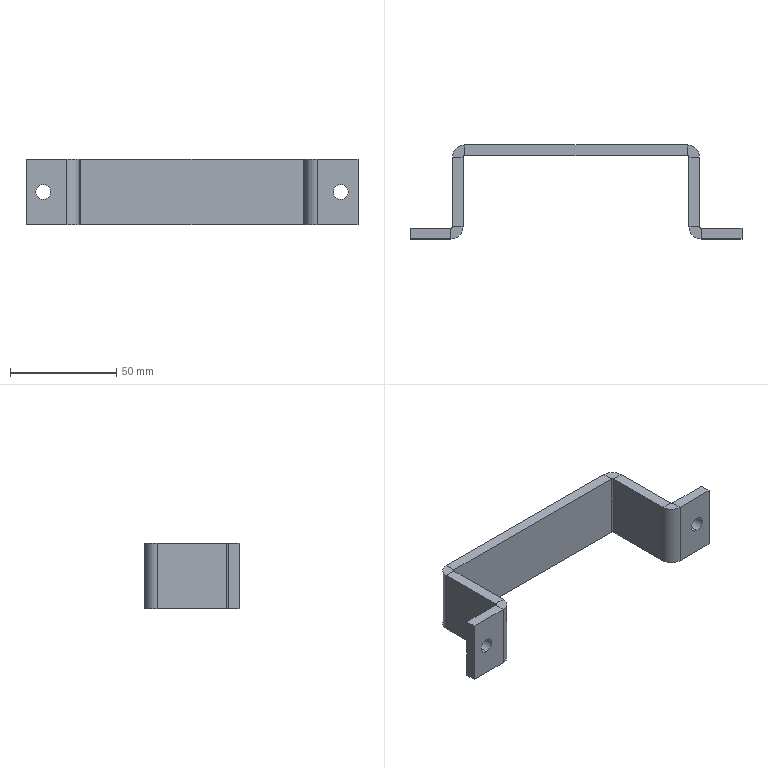Part | SolidWorks | features FlatPattern 1, ICE 1, SMBaseFlange 1, SheetMetal 1 | 1 solid | 42 faces | box 156.25 x 44.25 x 30.75 mm | volume 34854 mm3 | plane 30 | cylinder 12 | commonest cylinder face diameters 1.473 x4 7 x4 11.473 x4
STEP:
#1=CARTESIAN_POINT('',(-70.,-44.25,3.5));
#2=VERTEX_POINT('',#1);
#3=CARTESIAN_POINT('',(-70.,-44.25,-3.5));
#4=VERTEX_POINT('',#3);
#5=CARTESIAN_POINT('',(-70.,-44.25,0.));
#6=DIRECTION('',(0.,-1.,0.));
#7=DIRECTION('',(0.,0.,-1.));
#8=AXIS2_PLACEMENT_3D('',#5,#6,#7);
#9=CIRCLE('',#8,3.5);
#10=EDGE_CURVE('',#2,#4,#9,.T.);
#11=ORIENTED_EDGE('',*,*,#10,.T.);
#12=CARTESIAN_POINT('',(-70.,-39.25,-3.5));
#13=VERTEX_POINT('',#12);
#14=CARTESIAN_POINT('',(-70.,-49.25,-3.5));
#15=DIRECTION('',(0.,1.,0.));
#16=VECTOR('',#15,1000.);
#17=LINE('',#14,#16);
#18=EDGE_CURVE('',#4,#13,#17,.T.);
#19=ORIENTED_EDGE('',*,*,#18,.T.);
#20=CARTESIAN_POINT('',(-70.,-39.25,3.5));
#21=VERTEX_POINT('',#20);
#22=CARTESIAN_POINT('',(-70.,-39.25,0.));
#23=DIRECTION('',(0.,1.,0.));
#24=DIRECTION('',(0.,0.,1.));
#25=AXIS2_PLACEMENT_3D('',#22,#23,#24);
#26=CIRCLE('',#25,3.5);
#27=EDGE_CURVE('',#13,#21,#26,.T.);
#28=ORIENTED_EDGE('',*,*,#27,.T.);
#29=CARTESIAN_POINT('',(-70.,-49.25,3.5));
#30=DIRECTION('',(0.,1.,0.));
#31=VECTOR('',#30,1000.);
#32=LINE('',#29,#31);
#33=EDGE_CURVE('',#2,#21,#32,.T.);
#34=ORIENTED_EDGE('',*,*,#33,.F.);
#35=EDGE_LOOP('',(#11,#19,#28,#34));
#36=FACE_OUTER_BOUND('',#35,.T.);
#37=CARTESIAN_POINT('',(-70.,-49.25,0.));
#38=DIRECTION('',(0.,1.,0.));
#39=DIRECTION('',(0.,0.,1.));
#40=AXIS2_PLACEMENT_3D('',#37,#38,#39);
#41=CYLINDRICAL_SURFACE('',#40,3.5);
#42=ADVANCED_FACE('',(#36),#41,.F.);
#43=CARTESIAN_POINT('',(70.,-44.25,3.5));
#44=VERTEX_POINT('',#43);
#45=CARTESIAN_POINT('',(70.,-44.25,-3.5));
#46=VERTEX_POINT('',#45);
#47=CARTESIAN_POINT('',(70.,-44.25,0.));
#48=DIRECTION('',(0.,-1.,0.));
#49=DIRECTION('',(0.,0.,-1.));
#50=AXIS2_PLACEMENT_3D('',#47,#48,#49);
#51=CIRCLE('',#50,3.5);
#52=EDGE_CURVE('',#44,#46,#51,.T.);
#53=ORIENTED_EDGE('',*,*,#52,.T.);
#54=CARTESIAN_POINT('',(70.,-39.25,-3.5));
#55=VERTEX_POINT('',#54);
#56=CARTESIAN_POINT('',(70.,-49.25,-3.5));
#57=DIRECTION('',(0.,1.,0.));
#58=VECTOR('',#57,1000.);
#59=LINE('',#56,#58);
#60=EDGE_CURVE('',#46,#55,#59,.T.);
#61=ORIENTED_EDGE('',*,*,#60,.T.);
#62=CARTESIAN_POINT('',(70.,-39.25,3.5));
#63=VERTEX_POINT('',#62);
#64=CARTESIAN_POINT('',(70.,-39.25,0.));
#65=DIRECTION('',(0.,1.,0.));
#66=DIRECTION('',(0.,0.,1.));
#67=AXIS2_PLACEMENT_3D('',#64,#65,#66);
#68=CIRCLE('',#67,3.5);
#69=EDGE_CURVE('',#55,#63,#68,.T.);
#70=ORIENTED_EDGE('',*,*,#69,.T.);
#71=CARTESIAN_POINT('',(70.,-49.25,3.5));
#72=DIRECTION('',(0.,1.,0.));
#73=VECTOR('',#72,1000.);
#74=LINE('',#71,#73);
#75=EDGE_CURVE('',#44,#63,#74,.T.);
#76=ORIENTED_EDGE('',*,*,#75,.F.);
#77=EDGE_LOOP('',(#53,#61,#70,#76));
#78=FACE_OUTER_BOUND('',#77,.T.);
#79=CARTESIAN_POINT('',(70.,-49.25,0.));
#80=DIRECTION('',(0.,1.,0.));
#81=DIRECTION('',(0.,0.,1.));
#82=AXIS2_PLACEMENT_3D('',#79,#80,#81);
#83=CYLINDRICAL_SURFACE('',#82,3.5);
#84=ADVANCED_FACE('',(#78),#83,.F.);
#85=CARTESIAN_POINT('',(58.862,-39.25,15.375));
#86=VERTEX_POINT('',#85);
#87=CARTESIAN_POINT('',(58.862,-44.25,15.375));
#88=VERTEX_POINT('',#87);
#89=CARTESIAN_POINT('',(58.862,-39.25,15.375));
#90=DIRECTION('',(0.,-1.,0.));
#91=VECTOR('',#90,1000.);
#92=LINE('',#89,#91);
#93=EDGE_CURVE('',#86,#88,#92,.T.);
#94=ORIENTED_EDGE('',*,*,#93,.F.);
#95=CARTESIAN_POINT('',(58.125,-38.513,15.375));
#96=VERTEX_POINT('',#95);
#97=CARTESIAN_POINT('',(58.862,-38.513,15.375));
#98=DIRECTION('',(0.,0.,-1.));
#99=DIRECTION('',(1.,0.,0.));
#100=AXIS2_PLACEMENT_3D('',#97,#98,#99);
#101=CIRCLE('',#100,0.7366);
#102=EDGE_CURVE('',#86,#96,#101,.T.);
#103=ORIENTED_EDGE('',*,*,#102,.T.);
#104=CARTESIAN_POINT('',(53.125,-38.513,15.375));
#105=VERTEX_POINT('',#104);
#106=CARTESIAN_POINT('',(53.125,-38.513,15.375));
#107=DIRECTION('',(1.,0.,0.));
#108=VECTOR('',#107,1000.);
#109=LINE('',#106,#108);
#110=EDGE_CURVE('',#105,#96,#109,.T.);
#111=ORIENTED_EDGE('',*,*,#110,.F.);
#112=CARTESIAN_POINT('',(58.862,-38.513,15.375));
#113=DIRECTION('',(0.,0.,-1.));
#114=DIRECTION('',(1.,0.,0.));
#115=AXIS2_PLACEMENT_3D('',#112,#113,#114);
#116=CIRCLE('',#115,5.737);
#117=EDGE_CURVE('',#88,#105,#116,.T.);
#118=ORIENTED_EDGE('',*,*,#117,.F.);
#119=EDGE_LOOP('',(#94,#103,#111,#118));
#120=FACE_OUTER_BOUND('',#119,.T.);
#121=CARTESIAN_POINT('',(58.862,-39.25,15.375));
#122=DIRECTION('',(0.,0.,1.));
#123=DIRECTION('',(1.,0.,0.));
#124=AXIS2_PLACEMENT_3D('',#121,#122,#123);
#125=PLANE('',#124);
#126=ADVANCED_FACE('',(#120),#125,.T.);
#127=CARTESIAN_POINT('',(78.125,-39.25,15.375));
#128=VERTEX_POINT('',#127);
#129=CARTESIAN_POINT('',(58.125,-39.25,15.375));
#130=DIRECTION('',(-1.,0.,0.));
#131=VECTOR('',#130,1000.);
#132=LINE('',#129,#131);
#133=EDGE_CURVE('',#128,#86,#132,.T.);
#134=ORIENTED_EDGE('',*,*,#133,.T.);
#135=ORIENTED_EDGE('',*,*,#93,.T.);
#136=CARTESIAN_POINT('',(78.125,-44.25,15.375));
#137=VERTEX_POINT('',#136);
#138=CARTESIAN_POINT('',(58.125,-44.25,15.375));
#139=DIRECTION('',(-1.,0.,0.));
#140=VECTOR('',#139,1000.);
#141=LINE('',#138,#140);
#142=EDGE_CURVE('',#137,#88,#141,.T.);
#143=ORIENTED_EDGE('',*,*,#142,.F.);
#144=CARTESIAN_POINT('',(78.125,-39.25,15.375));
#145=DIRECTION('',(0.,-1.,0.));
#146=VECTOR('',#145,1000.);
#147=LINE('',#144,#146);
#148=EDGE_CURVE('',#128,#137,#147,.T.);
#149=ORIENTED_EDGE('',*,*,#148,.F.);
#150=EDGE_LOOP('',(#134,#135,#143,#149));
#151=FACE_OUTER_BOUND('',#150,.T.);
#152=CARTESIAN_POINT('',(53.125,-38.513,15.375));
#153=DIRECTION('',(0.,0.,1.));
#154=DIRECTION('',(1.,0.,0.));
#155=AXIS2_PLACEMENT_3D('',#152,#153,#154);
#156=PLANE('',#155);
#157=ADVANCED_FACE('',(#151),#156,.T.);
#158=CARTESIAN_POINT('',(58.125,-38.513,-15.375));
#159=VERTEX_POINT('',#158);
#160=CARTESIAN_POINT('',(53.125,-38.513,-15.375));
#161=VERTEX_POINT('',#160);
#162=CARTESIAN_POINT('',(58.125,-38.513,-15.375));
#163=DIRECTION('',(-1.,0.,0.));
#164=VECTOR('',#163,1000.);
#165=LINE('',#162,#164);
#166=EDGE_CURVE('',#159,#161,#165,.T.);
#167=ORIENTED_EDGE('',*,*,#166,.F.);
#168=CARTESIAN_POINT('',(58.862,-39.25,-15.375));
#169=VERTEX_POINT('',#168);
#170=CARTESIAN_POINT('',(58.862,-38.513,-15.375));
#171=DIRECTION('',(0.,0.,-1.));
#172=DIRECTION('',(1.,0.,0.));
#173=AXIS2_PLACEMENT_3D('',#170,#171,#172);
#174=CIRCLE('',#173,0.7366);
#175=EDGE_CURVE('',#169,#159,#174,.T.);
#176=ORIENTED_EDGE('',*,*,#175,.F.);
#177=CARTESIAN_POINT('',(58.862,-44.25,-15.375));
#178=VERTEX_POINT('',#177);
#179=CARTESIAN_POINT('',(58.862,-44.25,-15.375));
#180=DIRECTION('',(0.,1.,0.));
#181=VECTOR('',#180,1000.);
#182=LINE('',#179,#181);
#183=EDGE_CURVE('',#178,#169,#182,.T.);
#184=ORIENTED_EDGE('',*,*,#183,.F.);
#185=CARTESIAN_POINT('',(58.862,-38.513,-15.375));
#186=DIRECTION('',(0.,0.,-1.));
#187=DIRECTION('',(1.,0.,0.));
#188=AXIS2_PLACEMENT_3D('',#185,#186,#187);
#189=CIRCLE('',#188,5.737);
#190=EDGE_CURVE('',#178,#161,#189,.T.);
#191=ORIENTED_EDGE('',*,*,#190,.T.);
#192=EDGE_LOOP('',(#167,#176,#184,#191));
#193=FACE_OUTER_BOUND('',#192,.T.);
#194=CARTESIAN_POINT('',(58.125,-38.513,-15.375));
#195=DIRECTION('',(0.,0.,-1.));
#196=DIRECTION('',(-1.,0.,0.));
#197=AXIS2_PLACEMENT_3D('',#194,#195,#196);
#198=PLANE('',#197);
#199=ADVANCED_FACE('',(#193),#198,.T.);
#200=CARTESIAN_POINT('',(58.125,-5.737,-15.375));
#201=VERTEX_POINT('',#200);
#202=CARTESIAN_POINT('',(58.125,0.,-15.375));
#203=DIRECTION('',(0.,1.,0.));
#204=VECTOR('',#203,1000.);
#205=LINE('',#202,#204);
#206=EDGE_CURVE('',#159,#201,#205,.T.);
#207=ORIENTED_EDGE('',*,*,#206,.F.);
#208=ORIENTED_EDGE('',*,*,#166,.T.);
#209=CARTESIAN_POINT('',(53.125,-5.737,-15.375));
#210=VERTEX_POINT('',#209);
#211=CARTESIAN_POINT('',(53.125,0.,-15.375));
#212=DIRECTION('',(0.,1.,0.));
#213=VECTOR('',#212,1000.);
#214=LINE('',#211,#213);
#215=EDGE_CURVE('',#161,#210,#214,.T.);
#216=ORIENTED_EDGE('',*,*,#215,.T.);
#217=CARTESIAN_POINT('',(53.125,-5.737,-15.375));
#218=DIRECTION('',(1.,0.,0.));
#219=VECTOR('',#218,1000.);
#220=LINE('',#217,#219);
#221=EDGE_CURVE('',#210,#201,#220,.T.);
#222=ORIENTED_EDGE('',*,*,#221,.T.);
#223=EDGE_LOOP('',(#207,#208,#216,#222));
#224=FACE_OUTER_BOUND('',#223,.T.);
#225=CARTESIAN_POINT('',(58.862,-44.25,-15.375));
#226=DIRECTION('',(0.,0.,-1.));
#227=DIRECTION('',(-1.,0.,0.));
#228=AXIS2_PLACEMENT_3D('',#225,#226,#227);
#229=PLANE('',#228);
#230=ADVANCED_FACE('',(#224),#229,.T.);
#231=CARTESIAN_POINT('',(58.125,-5.737,15.375));
#232=VERTEX_POINT('',#231);
#233=CARTESIAN_POINT('',(53.125,-5.737,15.375));
#234=VERTEX_POINT('',#233);
#235=CARTESIAN_POINT('',(58.125,-5.737,15.375));
#236=DIRECTION('',(-1.,0.,0.));
#237=VECTOR('',#236,1000.);
#238=LINE('',#235,#237);
#239=EDGE_CURVE('',#232,#234,#238,.T.);
#240=ORIENTED_EDGE('',*,*,#239,.F.);
#241=CARTESIAN_POINT('',(52.388,0.,15.375));
#242=VERTEX_POINT('',#241);
#243=CARTESIAN_POINT('',(52.388,-5.737,15.375));
#244=DIRECTION('',(0.,0.,1.));
#245=DIRECTION('',(-1.,0.,0.));
#246=AXIS2_PLACEMENT_3D('',#243,#244,#245);
#247=CIRCLE('',#246,5.737);
#248=EDGE_CURVE('',#232,#242,#247,.T.);
#249=ORIENTED_EDGE('',*,*,#248,.T.);
#250=CARTESIAN_POINT('',(52.388,-5.,15.375));
#251=VERTEX_POINT('',#250);
#252=CARTESIAN_POINT('',(52.388,-5.,15.375));
#253=DIRECTION('',(0.,1.,0.));
#254=VECTOR('',#253,1000.);
#255=LINE('',#252,#254);
#256=EDGE_CURVE('',#251,#242,#255,.T.);
#257=ORIENTED_EDGE('',*,*,#256,.F.);
#258=CARTESIAN_POINT('',(52.388,-5.737,15.375));
#259=DIRECTION('',(0.,0.,1.));
#260=DIRECTION('',(1.,0.,0.));
#261=AXIS2_PLACEMENT_3D('',#258,#259,#260);
#262=CIRCLE('',#261,0.7366);
#263=EDGE_CURVE('',#234,#251,#262,.T.);
#264=ORIENTED_EDGE('',*,*,#263,.F.);
#265=EDGE_LOOP('',(#240,#249,#257,#264));
#266=FACE_OUTER_BOUND('',#265,.T.);
#267=CARTESIAN_POINT('',(58.125,-5.737,15.375));
#268=DIRECTION('',(0.,0.,1.));
#269=DIRECTION('',(1.,0.,0.));
#270=AXIS2_PLACEMENT_3D('',#267,#268,#269);
#271=PLANE('',#270);
#272=ADVANCED_FACE('',(#266),#271,.T.);
#273=CARTESIAN_POINT('',(58.125,0.,15.375));
#274=DIRECTION('',(0.,1.,0.));
#275=VECTOR('',#274,1000.);
#276=LINE('',#273,#275);
#277=EDGE_CURVE('',#96,#232,#276,.T.);
#278=ORIENTED_EDGE('',*,*,#277,.T.);
#279=ORIENTED_EDGE('',*,*,#239,.T.);
#280=CARTESIAN_POINT('',(53.125,0.,15.375));
#281=DIRECTION('',(0.,1.,0.));
#282=VECTOR('',#281,1000.);
#283=LINE('',#280,#282);
#284=EDGE_CURVE('',#105,#234,#283,.T.);
#285=ORIENTED_EDGE('',*,*,#284,.F.);
#286=ORIENTED_EDGE('',*,*,#110,.T.);
#287=EDGE_LOOP('',(#278,#279,#285,#286));
#288=FACE_OUTER_BOUND('',#287,.T.);
#289=CARTESIAN_POINT('',(52.388,-5.,15.375));
#290=DIRECTION('',(0.,0.,1.));
#291=DIRECTION('',(1.,0.,0.));
#292=AXIS2_PLACEMENT_3D('',#289,#290,#291);
#293=PLANE('',#292);
#294=ADVANCED_FACE('',(#288),#293,.T.);
#295=CARTESIAN_POINT('',(52.388,0.,-15.375));
#296=VERTEX_POINT('',#295);
#297=CARTESIAN_POINT('',(52.388,-5.,-15.375));
#298=VERTEX_POINT('',#297);
#299=CARTESIAN_POINT('',(52.388,0.,-15.375));
#300=DIRECTION('',(0.,-1.,0.));
#301=VECTOR('',#300,1000.);
#302=LINE('',#299,#301);
#303=EDGE_CURVE('',#296,#298,#302,.T.);
#304=ORIENTED_EDGE('',*,*,#303,.F.);
#305=CARTESIAN_POINT('',(52.388,-5.737,-15.375));
#306=DIRECTION('',(0.,0.,1.));
#307=DIRECTION('',(-1.,0.,0.));
#308=AXIS2_PLACEMENT_3D('',#305,#306,#307);
#309=CIRCLE('',#308,5.737);
#310=EDGE_CURVE('',#201,#296,#309,.T.);
#311=ORIENTED_EDGE('',*,*,#310,.F.);
#312=ORIENTED_EDGE('',*,*,#221,.F.);
#313=CARTESIAN_POINT('',(52.388,-5.737,-15.375));
#314=DIRECTION('',(0.,0.,1.));
#315=DIRECTION('',(1.,0.,0.));
#316=AXIS2_PLACEMENT_3D('',#313,#314,#315);
#317=CIRCLE('',#316,0.7366);
#318=EDGE_CURVE('',#210,#298,#317,.T.);
#319=ORIENTED_EDGE('',*,*,#318,.T.);
#320=EDGE_LOOP('',(#304,#311,#312,#319));
#321=FACE_OUTER_BOUND('',#320,.T.);
#322=CARTESIAN_POINT('',(52.388,0.,-15.375));
#323=DIRECTION('',(0.,0.,-1.));
#324=DIRECTION('',(-1.,0.,0.));
#325=AXIS2_PLACEMENT_3D('',#322,#323,#324);
#326=PLANE('',#325);
#327=ADVANCED_FACE('',(#321),#326,.T.);
#328=CARTESIAN_POINT('',(-52.388,0.,-15.375));
#329=VERTEX_POINT('',#328);
#330=CARTESIAN_POINT('',(-58.125,0.,-15.375));
#331=DIRECTION('',(-1.,0.,0.));
#332=VECTOR('',#331,1000.);
#333=LINE('',#330,#332);
#334=EDGE_CURVE('',#296,#329,#333,.T.);
#335=ORIENTED_EDGE('',*,*,#334,.F.);
#336=ORIENTED_EDGE('',*,*,#303,.T.);
#337=CARTESIAN_POINT('',(-52.388,-5.,-15.375));
#338=VERTEX_POINT('',#337);
#339=CARTESIAN_POINT('',(-58.125,-5.,-15.375));
#340=DIRECTION('',(-1.,0.,0.));
#341=VECTOR('',#340,1000.);
#342=LINE('',#339,#341);
#343=EDGE_CURVE('',#298,#338,#342,.T.);
#344=ORIENTED_EDGE('',*,*,#343,.T.);
#345=CARTESIAN_POINT('',(-52.388,-5.,-15.375));
#346=DIRECTION('',(0.,1.,0.));
#347=VECTOR('',#346,1000.);
#348=LINE('',#345,#347);
#349=EDGE_CURVE('',#338,#329,#348,.T.);
#350=ORIENTED_EDGE('',*,*,#349,.T.);
#351=EDGE_LOOP('',(#335,#336,#344,#350));
#352=FACE_OUTER_BOUND('',#351,.T.);
#353=CARTESIAN_POINT('',(53.125,-5.737,-15.375));
#354=DIRECTION('',(0.,0.,-1.));
#355=DIRECTION('',(-1.,0.,0.));
#356=AXIS2_PLACEMENT_3D('',#353,#354,#355);
#357=PLANE('',#356);
#358=ADVANCED_FACE('',(#352),#357,.T.);
#359=CARTESIAN_POINT('',(-52.388,0.,15.375));
#360=VERTEX_POINT('',#359);
#361=CARTESIAN_POINT('',(-52.388,-5.,15.375));
#362=VERTEX_POINT('',#361);
#363=CARTESIAN_POINT('',(-52.388,0.,15.375));
#364=DIRECTION('',(0.,-1.,0.));
#365=VECTOR('',#364,1000.);
#366=LINE('',#363,#365);
#367=EDGE_CURVE('',#360,#362,#366,.T.);
#368=ORIENTED_EDGE('',*,*,#367,.F.);
#369=CARTESIAN_POINT('',(-58.125,-5.737,15.375));
#370=VERTEX_POINT('',#369);
#371=CARTESIAN_POINT('',(-52.388,-5.737,15.375));
#372=DIRECTION('',(0.,0.,1.));
#373=DIRECTION('',(-1.,0.,0.));
#374=AXIS2_PLACEMENT_3D('',#371,#372,#373);
#375=CIRCLE('',#374,5.737);
#376=EDGE_CURVE('',#360,#370,#375,.T.);
#377=ORIENTED_EDGE('',*,*,#376,.T.);
#378=CARTESIAN_POINT('',(-53.125,-5.737,15.375));
#379=VERTEX_POINT('',#378);
#380=CARTESIAN_POINT('',(-53.125,-5.737,15.375));
#381=DIRECTION('',(-1.,0.,0.));
#382=VECTOR('',#381,1000.);
#383=LINE('',#380,#382);
#384=EDGE_CURVE('',#379,#370,#383,.T.);
#385=ORIENTED_EDGE('',*,*,#384,.F.);
#386=CARTESIAN_POINT('',(-52.388,-5.737,15.375));
#387=DIRECTION('',(0.,0.,1.));
#388=DIRECTION('',(1.,0.,0.));
#389=AXIS2_PLACEMENT_3D('',#386,#387,#388);
#390=CIRCLE('',#389,0.7366);
#391=EDGE_CURVE('',#362,#379,#390,.T.);
#392=ORIENTED_EDGE('',*,*,#391,.F.);
#393=EDGE_LOOP('',(#368,#377,#385,#392));
#394=FACE_OUTER_BOUND('',#393,.T.);
#395=CARTESIAN_POINT('',(-52.388,0.,15.375));
#396=DIRECTION('',(0.,0.,1.));
#397=DIRECTION('',(1.,0.,0.));
#398=AXIS2_PLACEMENT_3D('',#395,#396,#397);
#399=PLANE('',#398);
#400=ADVANCED_FACE('',(#394),#399,.T.);
#401=CARTESIAN_POINT('',(-58.125,0.,15.375));
#402=DIRECTION('',(-1.,0.,0.));
#403=VECTOR('',#402,1000.);
#404=LINE('',#401,#403);
#405=EDGE_CURVE('',#242,#360,#404,.T.);
#406=ORIENTED_EDGE('',*,*,#405,.T.);
#407=ORIENTED_EDGE('',*,*,#367,.T.);
#408=CARTESIAN_POINT('',(-58.125,-5.,15.375));
#409=DIRECTION('',(-1.,0.,0.));
#410=VECTOR('',#409,1000.);
#411=LINE('',#408,#410);
#412=EDGE_CURVE('',#251,#362,#411,.T.);
#413=ORIENTED_EDGE('',*,*,#412,.F.);
#414=ORIENTED_EDGE('',*,*,#256,.T.);
#415=EDGE_LOOP('',(#406,#407,#413,#414));
#416=FACE_OUTER_BOUND('',#415,.T.);
#417=CARTESIAN_POINT('',(-53.125,-5.737,15.375));
#418=DIRECTION('',(0.,0.,1.));
#419=DIRECTION('',(1.,0.,0.));
#420=AXIS2_PLACEMENT_3D('',#417,#418,#419);
#421=PLANE('',#420);
#422=ADVANCED_FACE('',(#416),#421,.T.);
#423=CARTESIAN_POINT('',(-58.125,-5.737,-15.375));
#424=VERTEX_POINT('',#423);
#425=CARTESIAN_POINT('',(-53.125,-5.737,-15.375));
#426=VERTEX_POINT('',#425);
#427=CARTESIAN_POINT('',(-58.125,-5.737,-15.375));
#428=DIRECTION('',(1.,0.,0.));
#429=VECTOR('',#428,1000.);
#430=LINE('',#427,#429);
#431=EDGE_CURVE('',#424,#426,#430,.T.);
#432=ORIENTED_EDGE('',*,*,#431,.F.);
#433=CARTESIAN_POINT('',(-52.388,-5.737,-15.375));
#434=DIRECTION('',(0.,0.,1.));
#435=DIRECTION('',(-1.,0.,0.));
#436=AXIS2_PLACEMENT_3D('',#433,#434,#435);
#437=CIRCLE('',#436,5.737);
#438=EDGE_CURVE('',#329,#424,#437,.T.);
#439=ORIENTED_EDGE('',*,*,#438,.F.);
#440=ORIENTED_EDGE('',*,*,#349,.F.);
#441=CARTESIAN_POINT('',(-52.388,-5.737,-15.375));
#442=DIRECTION('',(0.,0.,1.));
#443=DIRECTION('',(1.,0.,0.));
#444=AXIS2_PLACEMENT_3D('',#441,#442,#443);
#445=CIRCLE('',#444,0.7366);
#446=EDGE_CURVE('',#338,#426,#445,.T.);
#447=ORIENTED_EDGE('',*,*,#446,.T.);
#448=EDGE_LOOP('',(#432,#439,#440,#447));
#449=FACE_OUTER_BOUND('',#448,.T.);
#450=CARTESIAN_POINT('',(-58.125,-5.737,-15.375));
#451=DIRECTION('',(0.,0.,-1.));
#452=DIRECTION('',(-1.,0.,0.));
#453=AXIS2_PLACEMENT_3D('',#450,#451,#452);
#454=PLANE('',#453);
#455=ADVANCED_FACE('',(#449),#454,.T.);
#456=CARTESIAN_POINT('',(-58.125,-38.513,-15.375));
#457=VERTEX_POINT('',#456);
#458=CARTESIAN_POINT('',(-58.125,0.,-15.375));
#459=DIRECTION('',(0.,-1.,0.));
#460=VECTOR('',#459,1000.);
#461=LINE('',#458,#460);
#462=EDGE_CURVE('',#424,#457,#461,.T.);
#463=ORIENTED_EDGE('',*,*,#462,.F.);
#464=ORIENTED_EDGE('',*,*,#431,.T.);
#465=CARTESIAN_POINT('',(-53.125,-38.513,-15.375));
#466=VERTEX_POINT('',#465);
#467=CARTESIAN_POINT('',(-53.125,0.,-15.375));
#468=DIRECTION('',(0.,-1.,0.));
#469=VECTOR('',#468,1000.);
#470=LINE('',#467,#469);
#471=EDGE_CURVE('',#426,#466,#470,.T.);
#472=ORIENTED_EDGE('',*,*,#471,.T.);
#473=CARTESIAN_POINT('',(-53.125,-38.513,-15.375));
#474=DIRECTION('',(-1.,0.,0.));
#475=VECTOR('',#474,1000.);
#476=LINE('',#473,#475);
#477=EDGE_CURVE('',#466,#457,#476,.T.);
#478=ORIENTED_EDGE('',*,*,#477,.T.);
#479=EDGE_LOOP('',(#463,#464,#472,#478));
#480=FACE_OUTER_BOUND('',#479,.T.);
#481=CARTESIAN_POINT('',(-52.388,-5.,-15.375));
#482=DIRECTION('',(0.,0.,-1.));
#483=DIRECTION('',(-1.,0.,0.));
#484=AXIS2_PLACEMENT_3D('',#481,#482,#483);
#485=PLANE('',#484);
#486=ADVANCED_FACE('',(#480),#485,.T.);
#487=CARTESIAN_POINT('',(-58.125,-38.513,15.375));
#488=VERTEX_POINT('',#487);
#489=CARTESIAN_POINT('',(-53.125,-38.513,15.375));
#490=VERTEX_POINT('',#489);
#491=CARTESIAN_POINT('',(-58.125,-38.513,15.375));
#492=DIRECTION('',(1.,0.,0.));
#493=VECTOR('',#492,1000.);
#494=LINE('',#491,#493);
#495=EDGE_CURVE('',#488,#490,#494,.T.);
#496=ORIENTED_EDGE('',*,*,#495,.F.);
#497=CARTESIAN_POINT('',(-58.862,-39.25,15.375));
#498=VERTEX_POINT('',#497);
#499=CARTESIAN_POINT('',(-58.862,-38.513,15.375));
#500=DIRECTION('',(0.,0.,-1.));
#501=DIRECTION('',(1.,0.,0.));
#502=AXIS2_PLACEMENT_3D('',#499,#500,#501);
#503=CIRCLE('',#502,0.7366);
#504=EDGE_CURVE('',#488,#498,#503,.T.);
#505=ORIENTED_EDGE('',*,*,#504,.T.);
#506=CARTESIAN_POINT('',(-58.862,-44.25,15.375));
#507=VERTEX_POINT('',#506);
#508=CARTESIAN_POINT('',(-58.862,-44.25,15.375));
#509=DIRECTION('',(0.,1.,0.));
#510=VECTOR('',#509,1000.);
#511=LINE('',#508,#510);
#512=EDGE_CURVE('',#507,#498,#511,.T.);
#513=ORIENTED_EDGE('',*,*,#512,.F.);
#514=CARTESIAN_POINT('',(-58.862,-38.513,15.375));
#515=DIRECTION('',(0.,0.,-1.));
#516=DIRECTION('',(1.,0.,0.));
#517=AXIS2_PLACEMENT_3D('',#514,#515,#516);
#518=CIRCLE('',#517,5.737);
#519=EDGE_CURVE('',#490,#507,#518,.T.);
#520=ORIENTED_EDGE('',*,*,#519,.F.);
#521=EDGE_LOOP('',(#496,#505,#513,#520));
#522=FACE_OUTER_BOUND('',#521,.T.);
#523=CARTESIAN_POINT('',(-58.125,-38.513,15.375));
#524=DIRECTION('',(0.,0.,1.));
#525=DIRECTION('',(1.,0.,0.));
#526=AXIS2_PLACEMENT_3D('',#523,#524,#525);
#527=PLANE('',#526);
#528=ADVANCED_FACE('',(#522),#527,.T.);
#529=CARTESIAN_POINT('',(-58.125,0.,15.375));
#530=DIRECTION('',(0.,-1.,0.));
#531=VECTOR('',#530,1000.);
#532=LINE('',#529,#531);
#533=EDGE_CURVE('',#370,#488,#532,.T.);
#534=ORIENTED_EDGE('',*,*,#533,.T.);
#535=ORIENTED_EDGE('',*,*,#495,.T.);
#536=CARTESIAN_POINT('',(-53.125,0.,15.375));
#537=DIRECTION('',(0.,-1.,0.));
#538=VECTOR('',#537,1000.);
#539=LINE('',#536,#538);
#540=EDGE_CURVE('',#379,#490,#539,.T.);
#541=ORIENTED_EDGE('',*,*,#540,.F.);
#542=ORIENTED_EDGE('',*,*,#384,.T.);
#543=EDGE_LOOP('',(#534,#535,#541,#542));
#544=FACE_OUTER_BOUND('',#543,.T.);
#545=CARTESIAN_POINT('',(-58.862,-44.25,15.375));
#546=DIRECTION('',(0.,0.,1.));
#547=DIRECTION('',(1.,0.,0.));
#548=AXIS2_PLACEMENT_3D('',#545,#546,#547);
#549=PLANE('',#548);
#550=ADVANCED_FACE('',(#544),#549,.T.);
#551=CARTESIAN_POINT('',(-58.862,-39.25,-15.375));
#552=VERTEX_POINT('',#551);
#553=CARTESIAN_POINT('',(-58.862,-44.25,-15.375));
#554=VERTEX_POINT('',#553);
#555=CARTESIAN_POINT('',(-58.862,-39.25,-15.375));
#556=DIRECTION('',(0.,-1.,0.));
#557=VECTOR('',#556,1000.);
#558=LINE('',#555,#557);
#559=EDGE_CURVE('',#552,#554,#558,.T.);
#560=ORIENTED_EDGE('',*,*,#559,.F.);
#561=CARTESIAN_POINT('',(-58.862,-38.513,-15.375));
#562=DIRECTION('',(0.,0.,-1.));
#563=DIRECTION('',(1.,0.,0.));
#564=AXIS2_PLACEMENT_3D('',#561,#562,#563);
#565=CIRCLE('',#564,0.7366);
#566=EDGE_CURVE('',#457,#552,#565,.T.);
#567=ORIENTED_EDGE('',*,*,#566,.F.);
#568=ORIENTED_EDGE('',*,*,#477,.F.);
#569=CARTESIAN_POINT('',(-58.862,-38.513,-15.375));
#570=DIRECTION('',(0.,0.,-1.));
#571=DIRECTION('',(1.,0.,0.));
#572=AXIS2_PLACEMENT_3D('',#569,#570,#571);
#573=CIRCLE('',#572,5.737);
#574=EDGE_CURVE('',#466,#554,#573,.T.);
#575=ORIENTED_EDGE('',*,*,#574,.T.);
#576=EDGE_LOOP('',(#560,#567,#568,#575));
#577=FACE_OUTER_BOUND('',#576,.T.);
#578=CARTESIAN_POINT('',(-58.862,-39.25,-15.375));
#579=DIRECTION('',(0.,0.,-1.));
#580=DIRECTION('',(-1.,0.,0.));
#581=AXIS2_PLACEMENT_3D('',#578,#579,#580);
#582=PLANE('',#581);
#583=ADVANCED_FACE('',(#577),#582,.T.);
#584=CARTESIAN_POINT('',(-78.125,-39.25,-15.375));
#585=VERTEX_POINT('',#584);
#586=CARTESIAN_POINT('',(-58.125,-39.25,-15.375));
#587=DIRECTION('',(-1.,0.,0.));
#588=VECTOR('',#587,1000.);
#589=LINE('',#586,#588);
#590=EDGE_CURVE('',#552,#585,#589,.T.);
#591=ORIENTED_EDGE('',*,*,#590,.F.);
#592=ORIENTED_EDGE('',*,*,#559,.T.);
#593=CARTESIAN_POINT('',(-78.125,-44.25,-15.375));
#594=VERTEX_POINT('',#593);
#595=CARTESIAN_POINT('',(-58.125,-44.25,-15.375));
#596=DIRECTION('',(-1.,0.,0.));
#597=VECTOR('',#596,1000.);
#598=LINE('',#595,#597);
#599=EDGE_CURVE('',#554,#594,#598,.T.);
#600=ORIENTED_EDGE('',*,*,#599,.T.);
#601=CARTESIAN_POINT('',(-78.125,-44.25,-15.375));
#602=DIRECTION('',(0.,1.,0.));
#603=VECTOR('',#602,1000.);
#604=LINE('',#601,#603);
#605=EDGE_CURVE('',#594,#585,#604,.T.);
#606=ORIENTED_EDGE('',*,*,#605,.T.);
#607=EDGE_LOOP('',(#591,#592,#600,#606));
#608=FACE_OUTER_BOUND('',#607,.T.);
#609=CARTESIAN_POINT('',(-53.125,-38.513,-15.375));
#610=DIRECTION('',(0.,0.,-1.));
#611=DIRECTION('',(-1.,0.,0.));
#612=AXIS2_PLACEMENT_3D('',#609,#610,#611);
#613=PLANE('',#612);
#614=ADVANCED_FACE('',(#608),#613,.T.);
#615=CARTESIAN_POINT('',(-70.,-39.25,0.));
#616=DIRECTION('',(0.,1.,0.));
#617=DIRECTION('',(0.,0.,1.));
#618=AXIS2_PLACEMENT_3D('',#615,#616,#617);
#619=CIRCLE('',#618,3.5);
#620=EDGE_CURVE('',#21,#13,#619,.T.);
#621=ORIENTED_EDGE('',*,*,#620,.F.);
#622=ORIENTED_EDGE('',*,*,#27,.F.);
#623=EDGE_LOOP('',(#621,#622));
#624=FACE_BOUND('',#623,.T.);
#625=ORIENTED_EDGE('',*,*,#590,.T.);
#626=CARTESIAN_POINT('',(-78.125,-39.25,15.375));
#627=VERTEX_POINT('',#626);
#628=CARTESIAN_POINT('',(-78.125,-39.25,15.375));
#629=DIRECTION('',(0.,0.,-1.));
#630=VECTOR('',#629,1000.);
#631=LINE('',#628,#630);
#632=EDGE_CURVE('',#627,#585,#631,.T.);
#633=ORIENTED_EDGE('',*,*,#632,.F.);
#634=CARTESIAN_POINT('',(-58.125,-39.25,15.375));
#635=DIRECTION('',(-1.,0.,0.));
#636=VECTOR('',#635,1000.);
#637=LINE('',#634,#636);
#638=EDGE_CURVE('',#498,#627,#637,.T.);
#639=ORIENTED_EDGE('',*,*,#638,.F.);
#640=CARTESIAN_POINT('',(-58.862,-39.25,15.375));
#641=DIRECTION('',(0.,0.,-1.));
#642=VECTOR('',#641,1000.);
#643=LINE('',#640,#642);
#644=EDGE_CURVE('',#498,#552,#643,.T.);
#645=ORIENTED_EDGE('',*,*,#644,.T.);
#646=EDGE_LOOP('',(#625,#633,#639,#645));
#647=FACE_OUTER_BOUND('',#646,.T.);
#648=CARTESIAN_POINT('',(-58.125,-39.25,15.375));
#649=DIRECTION('',(0.,-1.,0.));
#650=DIRECTION('',(0.,0.,-1.));
#651=AXIS2_PLACEMENT_3D('',#648,#649,#650);
#652=PLANE('',#651);
#653=ADVANCED_FACE('',(#624,#647),#652,.F.);
#654=ORIENTED_EDGE('',*,*,#605,.F.);
#655=CARTESIAN_POINT('',(-78.125,-44.25,15.375));
#656=VERTEX_POINT('',#655);
#657=CARTESIAN_POINT('',(-78.125,-44.25,15.375));
#658=DIRECTION('',(0.,0.,-1.));
#659=VECTOR('',#658,1000.);
#660=LINE('',#657,#659);
#661=EDGE_CURVE('',#656,#594,#660,.T.);
#662=ORIENTED_EDGE('',*,*,#661,.F.);
#663=CARTESIAN_POINT('',(-78.125,-44.25,15.375));
#664=DIRECTION('',(0.,1.,0.));
#665=VECTOR('',#664,1000.);
#666=LINE('',#663,#665);
#667=EDGE_CURVE('',#656,#627,#666,.T.);
#668=ORIENTED_EDGE('',*,*,#667,.T.);
#669=ORIENTED_EDGE('',*,*,#632,.T.);
#670=EDGE_LOOP('',(#654,#662,#668,#669));
#671=FACE_OUTER_BOUND('',#670,.T.);
#672=CARTESIAN_POINT('',(-78.125,-44.25,15.375));
#673=DIRECTION('',(-1.,0.,0.));
#674=DIRECTION('',(0.,0.,1.));
#675=AXIS2_PLACEMENT_3D('',#672,#673,#674);
#676=PLANE('',#675);
#677=ADVANCED_FACE('',(#671),#676,.T.);
#678=ORIENTED_EDGE('',*,*,#10,.F.);
#679=CARTESIAN_POINT('',(-70.,-44.25,0.));
#680=DIRECTION('',(0.,-1.,0.));
#681=DIRECTION('',(0.,0.,-1.));
#682=AXIS2_PLACEMENT_3D('',#679,#680,#681);
#683=CIRCLE('',#682,3.5);
#684=EDGE_CURVE('',#4,#2,#683,.T.);
#685=ORIENTED_EDGE('',*,*,#684,.F.);
#686=EDGE_LOOP('',(#678,#685));
#687=FACE_BOUND('',#686,.T.);
#688=ORIENTED_EDGE('',*,*,#599,.F.);
#689=CARTESIAN_POINT('',(-58.862,-44.25,15.375));
#690=DIRECTION('',(0.,0.,-1.));
#691=VECTOR('',#690,1000.);
#692=LINE('',#689,#691);
#693=EDGE_CURVE('',#507,#554,#692,.T.);
#694=ORIENTED_EDGE('',*,*,#693,.F.);
#695=CARTESIAN_POINT('',(-58.125,-44.25,15.375));
#696=DIRECTION('',(-1.,0.,0.));
#697=VECTOR('',#696,1000.);
#698=LINE('',#695,#697);
#699=EDGE_CURVE('',#507,#656,#698,.T.);
#700=ORIENTED_EDGE('',*,*,#699,.T.);
#701=ORIENTED_EDGE('',*,*,#661,.T.);
#702=EDGE_LOOP('',(#688,#694,#700,#701));
#703=FACE_OUTER_BOUND('',#702,.T.);
#704=CARTESIAN_POINT('',(-58.125,-44.25,15.375));
#705=DIRECTION('',(0.,-1.,0.));
#706=DIRECTION('',(0.,0.,-1.));
#707=AXIS2_PLACEMENT_3D('',#704,#705,#706);
#708=PLANE('',#707);
#709=ADVANCED_FACE('',(#687,#703),#708,.T.);
#710=ORIENTED_EDGE('',*,*,#574,.F.);
#711=CARTESIAN_POINT('',(-53.125,-38.513,15.375));
#712=DIRECTION('',(0.,0.,-1.));
#713=VECTOR('',#712,1000.);
#714=LINE('',#711,#713);
#715=EDGE_CURVE('',#490,#466,#714,.T.);
#716=ORIENTED_EDGE('',*,*,#715,.F.);
#717=ORIENTED_EDGE('',*,*,#519,.T.);
#718=ORIENTED_EDGE('',*,*,#693,.T.);
#719=EDGE_LOOP('',(#710,#716,#717,#718));
#720=FACE_OUTER_BOUND('',#719,.T.);
#721=CARTESIAN_POINT('',(-58.862,-38.513,15.375));
#722=DIRECTION('',(0.,0.,-1.));
#723=DIRECTION('',(-1.,0.,0.));
#724=AXIS2_PLACEMENT_3D('',#721,#722,#723);
#725=CYLINDRICAL_SURFACE('',#724,5.737);
#726=ADVANCED_FACE('',(#720),#725,.T.);
#727=ORIENTED_EDGE('',*,*,#471,.F.);
#728=CARTESIAN_POINT('',(-53.125,-5.737,15.375));
#729=DIRECTION('',(0.,0.,-1.));
#730=VECTOR('',#729,1000.);
#731=LINE('',#728,#730);
#732=EDGE_CURVE('',#379,#426,#731,.T.);
#733=ORIENTED_EDGE('',*,*,#732,.F.);
#734=ORIENTED_EDGE('',*,*,#540,.T.);
#735=ORIENTED_EDGE('',*,*,#715,.T.);
#736=EDGE_LOOP('',(#727,#733,#734,#735));
#737=FACE_OUTER_BOUND('',#736,.T.);
#738=CARTESIAN_POINT('',(-53.125,0.,15.375));
#739=DIRECTION('',(1.,0.,0.));
#740=DIRECTION('',(0.,1.,0.));
#741=AXIS2_PLACEMENT_3D('',#738,#739,#740);
#742=PLANE('',#741);
#743=ADVANCED_FACE('',(#737),#742,.T.);
#744=ORIENTED_EDGE('',*,*,#446,.F.);
#745=CARTESIAN_POINT('',(-52.388,-5.,15.375));
#746=DIRECTION('',(0.,0.,-1.));
#747=VECTOR('',#746,1000.);
#748=LINE('',#745,#747);
#749=EDGE_CURVE('',#362,#338,#748,.T.);
#750=ORIENTED_EDGE('',*,*,#749,.F.);
#751=ORIENTED_EDGE('',*,*,#391,.T.);
#752=ORIENTED_EDGE('',*,*,#732,.T.);
#753=EDGE_LOOP('',(#744,#750,#751,#752));
#754=FACE_OUTER_BOUND('',#753,.T.);
#755=CARTESIAN_POINT('',(-52.388,-5.737,15.375));
#756=DIRECTION('',(0.,0.,-1.));
#757=DIRECTION('',(-1.,0.,0.));
#758=AXIS2_PLACEMENT_3D('',#755,#756,#757);
#759=CYLINDRICAL_SURFACE('',#758,0.7366);
#760=ADVANCED_FACE('',(#754),#759,.F.);
#761=ORIENTED_EDGE('',*,*,#343,.F.);
#762=CARTESIAN_POINT('',(52.388,-5.,15.375));
#763=DIRECTION('',(0.,0.,-1.));
#764=VECTOR('',#763,1000.);
#765=LINE('',#762,#764);
#766=EDGE_CURVE('',#251,#298,#765,.T.);
#767=ORIENTED_EDGE('',*,*,#766,.F.);
#768=ORIENTED_EDGE('',*,*,#412,.T.);
#769=ORIENTED_EDGE('',*,*,#749,.T.);
#770=EDGE_LOOP('',(#761,#767,#768,#769));
#771=FACE_OUTER_BOUND('',#770,.T.);
#772=CARTESIAN_POINT('',(-58.125,-5.,15.375));
#773=DIRECTION('',(0.,-1.,0.));
#774=DIRECTION('',(0.,0.,-1.));
#775=AXIS2_PLACEMENT_3D('',#772,#773,#774);
#776=PLANE('',#775);
#777=ADVANCED_FACE('',(#771),#776,.T.);
#778=ORIENTED_EDGE('',*,*,#318,.F.);
#779=CARTESIAN_POINT('',(53.125,-5.737,15.375));
#780=DIRECTION('',(0.,0.,-1.));
#781=VECTOR('',#780,1000.);
#782=LINE('',#779,#781);
#783=EDGE_CURVE('',#234,#210,#782,.T.);
#784=ORIENTED_EDGE('',*,*,#783,.F.);
#785=ORIENTED_EDGE('',*,*,#263,.T.);
#786=ORIENTED_EDGE('',*,*,#766,.T.);
#787=EDGE_LOOP('',(#778,#784,#785,#786));
#788=FACE_OUTER_BOUND('',#787,.T.);
#789=CARTESIAN_POINT('',(52.388,-5.737,15.375));
#790=DIRECTION('',(0.,0.,-1.));
#791=DIRECTION('',(-1.,0.,0.));
#792=AXIS2_PLACEMENT_3D('',#789,#790,#791);
#793=CYLINDRICAL_SURFACE('',#792,0.7366);
#794=ADVANCED_FACE('',(#788),#793,.F.);
#795=ORIENTED_EDGE('',*,*,#215,.F.);
#796=CARTESIAN_POINT('',(53.125,-38.513,15.375));
#797=DIRECTION('',(0.,0.,-1.));
#798=VECTOR('',#797,1000.);
#799=LINE('',#796,#798);
#800=EDGE_CURVE('',#105,#161,#799,.T.);
#801=ORIENTED_EDGE('',*,*,#800,.F.);
#802=ORIENTED_EDGE('',*,*,#284,.T.);
#803=ORIENTED_EDGE('',*,*,#783,.T.);
#804=EDGE_LOOP('',(#795,#801,#802,#803));
#805=FACE_OUTER_BOUND('',#804,.T.);
#806=CARTESIAN_POINT('',(53.125,0.,15.375));
#807=DIRECTION('',(-1.,0.,0.));
#808=DIRECTION('',(0.,-1.,0.));
#809=AXIS2_PLACEMENT_3D('',#806,#807,#808);
#810=PLANE('',#809);
#811=ADVANCED_FACE('',(#805),#810,.T.);
#812=ORIENTED_EDGE('',*,*,#190,.F.);
#813=CARTESIAN_POINT('',(58.862,-44.25,15.375));
#814=DIRECTION('',(0.,0.,-1.));
#815=VECTOR('',#814,1000.);
#816=LINE('',#813,#815);
#817=EDGE_CURVE('',#88,#178,#816,.T.);
#818=ORIENTED_EDGE('',*,*,#817,.F.);
#819=ORIENTED_EDGE('',*,*,#117,.T.);
#820=ORIENTED_EDGE('',*,*,#800,.T.);
#821=EDGE_LOOP('',(#812,#818,#819,#820));
#822=FACE_OUTER_BOUND('',#821,.T.);
#823=CARTESIAN_POINT('',(58.862,-38.513,15.375));
#824=DIRECTION('',(0.,0.,-1.));
#825=DIRECTION('',(-1.,0.,0.));
#826=AXIS2_PLACEMENT_3D('',#823,#824,#825);
#827=CYLINDRICAL_SURFACE('',#826,5.737);
#828=ADVANCED_FACE('',(#822),#827,.T.);
#829=ORIENTED_EDGE('',*,*,#52,.F.);
#830=CARTESIAN_POINT('',(70.,-44.25,0.));
#831=DIRECTION('',(0.,-1.,0.));
#832=DIRECTION('',(0.,0.,-1.));
#833=AXIS2_PLACEMENT_3D('',#830,#831,#832);
#834=CIRCLE('',#833,3.5);
#835=EDGE_CURVE('',#46,#44,#834,.T.);
#836=ORIENTED_EDGE('',*,*,#835,.F.);
#837=EDGE_LOOP('',(#829,#836));
#838=FACE_BOUND('',#837,.T.);
#839=CARTESIAN_POINT('',(78.125,-44.25,-15.375));
#840=VERTEX_POINT('',#839);
#841=CARTESIAN_POINT('',(58.125,-44.25,-15.375));
#842=DIRECTION('',(-1.,0.,0.));
#843=VECTOR('',#842,1000.);
#844=LINE('',#841,#843);
#845=EDGE_CURVE('',#840,#178,#844,.T.);
#846=ORIENTED_EDGE('',*,*,#845,.F.);
#847=CARTESIAN_POINT('',(78.125,-44.25,15.375));
#848=DIRECTION('',(0.,0.,-1.));
#849=VECTOR('',#848,1000.);
#850=LINE('',#847,#849);
#851=EDGE_CURVE('',#137,#840,#850,.T.);
#852=ORIENTED_EDGE('',*,*,#851,.F.);
#853=ORIENTED_EDGE('',*,*,#142,.T.);
#854=ORIENTED_EDGE('',*,*,#817,.T.);
#855=EDGE_LOOP('',(#846,#852,#853,#854));
#856=FACE_OUTER_BOUND('',#855,.T.);
#857=CARTESIAN_POINT('',(58.125,-44.25,15.375));
#858=DIRECTION('',(0.,-1.,0.));
#859=DIRECTION('',(0.,0.,-1.));
#860=AXIS2_PLACEMENT_3D('',#857,#858,#859);
#861=PLANE('',#860);
#862=ADVANCED_FACE('',(#838,#856),#861,.T.);
#863=CARTESIAN_POINT('',(78.125,-39.25,-15.375));
#864=VERTEX_POINT('',#863);
#865=CARTESIAN_POINT('',(78.125,-39.25,-15.375));
#866=DIRECTION('',(0.,-1.,0.));
#867=VECTOR('',#866,1000.);
#868=LINE('',#865,#867);
#869=EDGE_CURVE('',#864,#840,#868,.T.);
#870=ORIENTED_EDGE('',*,*,#869,.F.);
#871=CARTESIAN_POINT('',(78.125,-39.25,15.375));
#872=DIRECTION('',(0.,0.,-1.));
#873=VECTOR('',#872,1000.);
#874=LINE('',#871,#873);
#875=EDGE_CURVE('',#128,#864,#874,.T.);
#876=ORIENTED_EDGE('',*,*,#875,.F.);
#877=ORIENTED_EDGE('',*,*,#148,.T.);
#878=ORIENTED_EDGE('',*,*,#851,.T.);
#879=EDGE_LOOP('',(#870,#876,#877,#878));
#880=FACE_OUTER_BOUND('',#879,.T.);
#881=CARTESIAN_POINT('',(78.125,-39.25,15.375));
#882=DIRECTION('',(1.,0.,0.));
#883=DIRECTION('',(0.,0.,-1.));
#884=AXIS2_PLACEMENT_3D('',#881,#882,#883);
#885=PLANE('',#884);
#886=ADVANCED_FACE('',(#880),#885,.T.);
#887=CARTESIAN_POINT('',(70.,-39.25,0.));
#888=DIRECTION('',(0.,1.,0.));
#889=DIRECTION('',(0.,0.,1.));
#890=AXIS2_PLACEMENT_3D('',#887,#888,#889);
#891=CIRCLE('',#890,3.5);
#892=EDGE_CURVE('',#63,#55,#891,.T.);
#893=ORIENTED_EDGE('',*,*,#892,.F.);
#894=ORIENTED_EDGE('',*,*,#69,.F.);
#895=EDGE_LOOP('',(#893,#894));
#896=FACE_BOUND('',#895,.T.);
#897=CARTESIAN_POINT('',(58.125,-39.25,-15.375));
#898=DIRECTION('',(-1.,0.,0.));
#899=VECTOR('',#898,1000.);
#900=LINE('',#897,#899);
#901=EDGE_CURVE('',#864,#169,#900,.T.);
#902=ORIENTED_EDGE('',*,*,#901,.T.);
#903=CARTESIAN_POINT('',(58.862,-39.25,15.375));
#904=DIRECTION('',(0.,0.,-1.));
#905=VECTOR('',#904,1000.);
#906=LINE('',#903,#905);
#907=EDGE_CURVE('',#86,#169,#906,.T.);
#908=ORIENTED_EDGE('',*,*,#907,.F.);
#909=ORIENTED_EDGE('',*,*,#133,.F.);
#910=ORIENTED_EDGE('',*,*,#875,.T.);
#911=EDGE_LOOP('',(#902,#908,#909,#910));
#912=FACE_OUTER_BOUND('',#911,.T.);
#913=CARTESIAN_POINT('',(58.125,-39.25,15.375));
#914=DIRECTION('',(0.,-1.,0.));
#915=DIRECTION('',(0.,0.,-1.));
#916=AXIS2_PLACEMENT_3D('',#913,#914,#915);
#917=PLANE('',#916);
#918=ADVANCED_FACE('',(#896,#912),#917,.F.);
#919=ORIENTED_EDGE('',*,*,#175,.T.);
#920=CARTESIAN_POINT('',(58.125,-38.513,15.375));
#921=DIRECTION('',(0.,0.,-1.));
#922=VECTOR('',#921,1000.);
#923=LINE('',#920,#922);
#924=EDGE_CURVE('',#96,#159,#923,.T.);
#925=ORIENTED_EDGE('',*,*,#924,.F.);
#926=ORIENTED_EDGE('',*,*,#102,.F.);
#927=ORIENTED_EDGE('',*,*,#907,.T.);
#928=EDGE_LOOP('',(#919,#925,#926,#927));
#929=FACE_OUTER_BOUND('',#928,.T.);
#930=CARTESIAN_POINT('',(58.862,-38.513,15.375));
#931=DIRECTION('',(0.,0.,-1.));
#932=DIRECTION('',(-1.,0.,0.));
#933=AXIS2_PLACEMENT_3D('',#930,#931,#932);
#934=CYLINDRICAL_SURFACE('',#933,0.7366);
#935=ADVANCED_FACE('',(#929),#934,.F.);
#936=ORIENTED_EDGE('',*,*,#206,.T.);
#937=CARTESIAN_POINT('',(58.125,-5.737,15.375));
#938=DIRECTION('',(0.,0.,-1.));
#939=VECTOR('',#938,1000.);
#940=LINE('',#937,#939);
#941=EDGE_CURVE('',#232,#201,#940,.T.);
#942=ORIENTED_EDGE('',*,*,#941,.F.);
#943=ORIENTED_EDGE('',*,*,#277,.F.);
#944=ORIENTED_EDGE('',*,*,#924,.T.);
#945=EDGE_LOOP('',(#936,#942,#943,#944));
#946=FACE_OUTER_BOUND('',#945,.T.);
#947=CARTESIAN_POINT('',(58.125,0.,15.375));
#948=DIRECTION('',(-1.,0.,0.));
#949=DIRECTION('',(0.,-1.,0.));
#950=AXIS2_PLACEMENT_3D('',#947,#948,#949);
#951=PLANE('',#950);
#952=ADVANCED_FACE('',(#946),#951,.F.);
#953=ORIENTED_EDGE('',*,*,#310,.T.);
#954=CARTESIAN_POINT('',(52.388,0.,15.375));
#955=DIRECTION('',(0.,0.,-1.));
#956=VECTOR('',#955,1000.);
#957=LINE('',#954,#956);
#958=EDGE_CURVE('',#242,#296,#957,.T.);
#959=ORIENTED_EDGE('',*,*,#958,.F.);
#960=ORIENTED_EDGE('',*,*,#248,.F.);
#961=ORIENTED_EDGE('',*,*,#941,.T.);
#962=EDGE_LOOP('',(#953,#959,#960,#961));
#963=FACE_OUTER_BOUND('',#962,.T.);
#964=CARTESIAN_POINT('',(52.388,-5.737,15.375));
#965=DIRECTION('',(0.,0.,-1.));
#966=DIRECTION('',(-1.,0.,0.));
#967=AXIS2_PLACEMENT_3D('',#964,#965,#966);
#968=CYLINDRICAL_SURFACE('',#967,5.737);
#969=ADVANCED_FACE('',(#963),#968,.T.);
#970=ORIENTED_EDGE('',*,*,#334,.T.);
#971=CARTESIAN_POINT('',(-52.388,0.,15.375));
#972=DIRECTION('',(0.,0.,-1.));
#973=VECTOR('',#972,1000.);
#974=LINE('',#971,#973);
#975=EDGE_CURVE('',#360,#329,#974,.T.);
#976=ORIENTED_EDGE('',*,*,#975,.F.);
#977=ORIENTED_EDGE('',*,*,#405,.F.);
#978=ORIENTED_EDGE('',*,*,#958,.T.);
#979=EDGE_LOOP('',(#970,#976,#977,#978));
#980=FACE_OUTER_BOUND('',#979,.T.);
#981=CARTESIAN_POINT('',(-58.125,0.,15.375));
#982=DIRECTION('',(0.,-1.,0.));
#983=DIRECTION('',(0.,0.,-1.));
#984=AXIS2_PLACEMENT_3D('',#981,#982,#983);
#985=PLANE('',#984);
#986=ADVANCED_FACE('',(#980),#985,.F.);
#987=ORIENTED_EDGE('',*,*,#438,.T.);
#988=CARTESIAN_POINT('',(-58.125,-5.737,15.375));
#989=DIRECTION('',(0.,0.,-1.));
#990=VECTOR('',#989,1000.);
#991=LINE('',#988,#990);
#992=EDGE_CURVE('',#370,#424,#991,.T.);
#993=ORIENTED_EDGE('',*,*,#992,.F.);
#994=ORIENTED_EDGE('',*,*,#376,.F.);
#995=ORIENTED_EDGE('',*,*,#975,.T.);
#996=EDGE_LOOP('',(#987,#993,#994,#995));
#997=FACE_OUTER_BOUND('',#996,.T.);
#998=CARTESIAN_POINT('',(-52.388,-5.737,15.375));
#999=DIRECTION('',(0.,0.,-1.));
#1000=DIRECTION('',(-1.,0.,0.));
#1001=AXIS2_PLACEMENT_3D('',#998,#999,#1000);
#1002=CYLINDRICAL_SURFACE('',#1001,5.737);
#1003=ADVANCED_FACE('',(#997),#1002,.T.);
#1004=ORIENTED_EDGE('',*,*,#462,.T.);
#1005=CARTESIAN_POINT('',(-58.125,-38.513,15.375));
#1006=DIRECTION('',(0.,0.,-1.));
#1007=VECTOR('',#1006,1000.);
#1008=LINE('',#1005,#1007);
#1009=EDGE_CURVE('',#488,#457,#1008,.T.);
#1010=ORIENTED_EDGE('',*,*,#1009,.F.);
#1011=ORIENTED_EDGE('',*,*,#533,.F.);
#1012=ORIENTED_EDGE('',*,*,#992,.T.);
#1013=EDGE_LOOP('',(#1004,#1010,#1011,#1012));
#1014=FACE_OUTER_BOUND('',#1013,.T.);
#1015=CARTESIAN_POINT('',(-58.125,0.,15.375));
#1016=DIRECTION('',(1.,0.,0.));
#1017=DIRECTION('',(0.,1.,0.));
#1018=AXIS2_PLACEMENT_3D('',#1015,#1016,#1017);
#1019=PLANE('',#1018);
#1020=ADVANCED_FACE('',(#1014),#1019,.F.);
#1021=ORIENTED_EDGE('',*,*,#566,.T.);
#1022=ORIENTED_EDGE('',*,*,#644,.F.);
#1023=ORIENTED_EDGE('',*,*,#504,.F.);
#1024=ORIENTED_EDGE('',*,*,#1009,.T.);
#1025=EDGE_LOOP('',(#1021,#1022,#1023,#1024));
#1026=FACE_OUTER_BOUND('',#1025,.T.);
#1027=CARTESIAN_POINT('',(-58.862,-38.513,15.375));
#1028=DIRECTION('',(0.,0.,-1.));
#1029=DIRECTION('',(-1.,0.,0.));
#1030=AXIS2_PLACEMENT_3D('',#1027,#1028,#1029);
#1031=CYLINDRICAL_SURFACE('',#1030,0.7366);
#1032=ADVANCED_FACE('',(#1026),#1031,.F.);
#1033=ORIENTED_EDGE('',*,*,#638,.T.);
#1034=ORIENTED_EDGE('',*,*,#667,.F.);
#1035=ORIENTED_EDGE('',*,*,#699,.F.);
#1036=ORIENTED_EDGE('',*,*,#512,.T.);
#1037=EDGE_LOOP('',(#1033,#1034,#1035,#1036));
#1038=FACE_OUTER_BOUND('',#1037,.T.);
#1039=CARTESIAN_POINT('',(-58.862,-38.513,15.375));
#1040=DIRECTION('',(0.,0.,1.));
#1041=DIRECTION('',(1.,0.,0.));
#1042=AXIS2_PLACEMENT_3D('',#1039,#1040,#1041);
#1043=PLANE('',#1042);
#1044=ADVANCED_FACE('',(#1038),#1043,.T.);
#1045=ORIENTED_EDGE('',*,*,#845,.T.);
#1046=ORIENTED_EDGE('',*,*,#183,.T.);
#1047=ORIENTED_EDGE('',*,*,#901,.F.);
#1048=ORIENTED_EDGE('',*,*,#869,.T.);
#1049=EDGE_LOOP('',(#1045,#1046,#1047,#1048));
#1050=FACE_OUTER_BOUND('',#1049,.T.);
#1051=CARTESIAN_POINT('',(-58.862,-38.513,-15.375));
#1052=DIRECTION('',(0.,0.,1.));
#1053=DIRECTION('',(1.,0.,0.));
#1054=AXIS2_PLACEMENT_3D('',#1051,#1052,#1053);
#1055=PLANE('',#1054);
#1056=ADVANCED_FACE('',(#1050),#1055,.F.);
#1057=ORIENTED_EDGE('',*,*,#60,.F.);
#1058=ORIENTED_EDGE('',*,*,#835,.T.);
#1059=ORIENTED_EDGE('',*,*,#75,.T.);
#1060=ORIENTED_EDGE('',*,*,#892,.T.);
#1061=EDGE_LOOP('',(#1057,#1058,#1059,#1060));
#1062=FACE_OUTER_BOUND('',#1061,.T.);
#1063=CARTESIAN_POINT('',(70.,-49.25,0.));
#1064=DIRECTION('',(0.,1.,0.));
#1065=DIRECTION('',(0.,0.,1.));
#1066=AXIS2_PLACEMENT_3D('',#1063,#1064,#1065);
#1067=CYLINDRICAL_SURFACE('',#1066,3.5);
#1068=ADVANCED_FACE('',(#1062),#1067,.F.);
#1069=ORIENTED_EDGE('',*,*,#18,.F.);
#1070=ORIENTED_EDGE('',*,*,#684,.T.);
#1071=ORIENTED_EDGE('',*,*,#33,.T.);
#1072=ORIENTED_EDGE('',*,*,#620,.T.);
#1073=EDGE_LOOP('',(#1069,#1070,#1071,#1072));
#1074=FACE_OUTER_BOUND('',#1073,.T.);
#1075=CARTESIAN_POINT('',(-70.,-49.25,0.));
#1076=DIRECTION('',(0.,1.,0.));
#1077=DIRECTION('',(0.,0.,1.));
#1078=AXIS2_PLACEMENT_3D('',#1075,#1076,#1077);
#1079=CYLINDRICAL_SURFACE('',#1078,3.5);
#1080=ADVANCED_FACE('',(#1074),#1079,.F.);
#1081=CLOSED_SHELL('',(#42,#84,#126,#157,#199,#230,#272,#294,#327,#358,#400,#422,#455,#486,#528,#550,#583,#614,#653,#677,#709,#726,#743,#760,#777,#794,#811,#828,#862,#886,#918,#935,#952,#969,#986,#1003,#1020,#1032,#1044,#1056,#1068,#1080));
#1082=MANIFOLD_SOLID_BREP('',#1081);
#1083=CARTESIAN_POINT('',(0.,0.,0.));
#1084=DIRECTION('',(0.,0.,1.));
#1085=DIRECTION('',(1.,0.,0.));
#1086=AXIS2_PLACEMENT_3D('',#1083,#1084,#1085);
#1087=(LENGTH_UNIT()NAMED_UNIT(*)SI_UNIT(.MILLI.,.METRE.));
#1088=UNCERTAINTY_MEASURE_WITH_UNIT(LENGTH_MEASURE(0.00001),#1087,'','');
#1089=(NAMED_UNIT(*)PLANE_ANGLE_UNIT()SI_UNIT($,.RADIAN.));
#1090=(NAMED_UNIT(*)SI_UNIT($,.STERADIAN.)SOLID_ANGLE_UNIT());
#1091=(GEOMETRIC_REPRESENTATION_CONTEXT(3)GLOBAL_UNCERTAINTY_ASSIGNED_CONTEXT((#1088))GLOBAL_UNIT_ASSIGNED_CONTEXT((#1087,#1089,#1090))REPRESENTATION_CONTEXT('',''));
#1092=ADVANCED_BREP_SHAPE_REPRESENTATION('',(#1082,#1086),#1091);